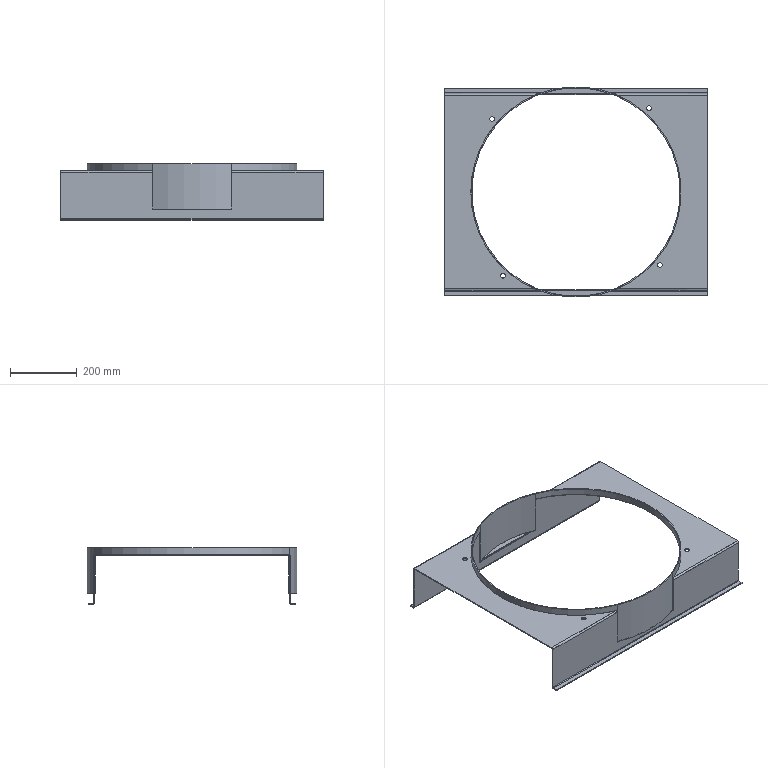Part | STEP file | Produce dryer cooling section-HY-40-M-601 | 7 solids | 97 faces | box 786 x 630 x 168 mm | volume 1349163 mm3 | plane 60 | cylinder 33 | spline 4 | commonest cylinder face diameters 14 x8 630 x7 4 x6 10 x6 624 x6